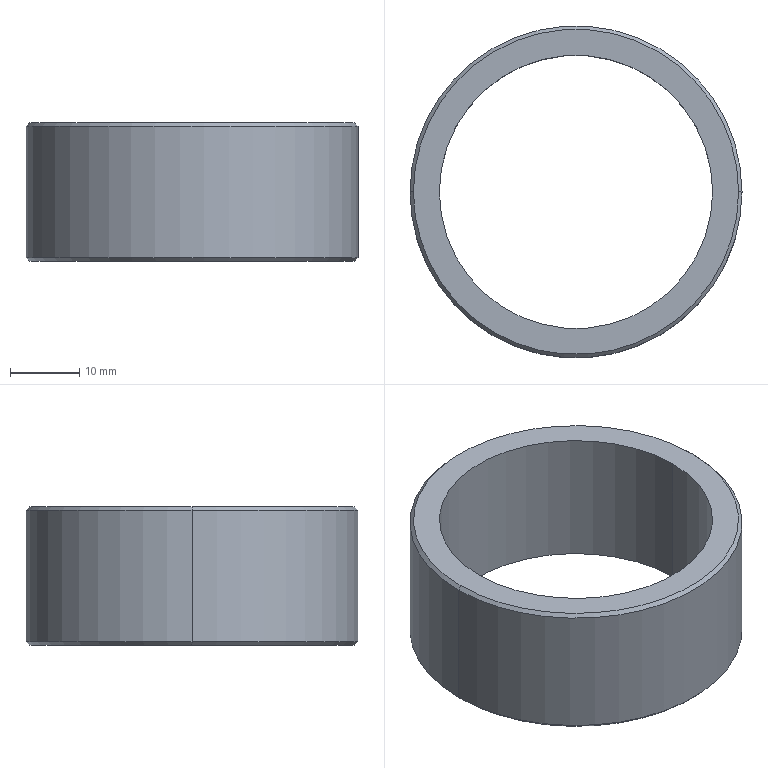Part | SolidWorks | features Chamfer 1, Extrusion 1 | 1 solid | 10 faces | box 48 x 48 x 20 mm | volume 11645 mm3 | cone 4 | cylinder 4 | plane 2 | commonest cylinder face diameters 39.5 x2 48 x2
STEP:
#1=CARTESIAN_POINT('',(23.5,0.,10.));
#2=VERTEX_POINT('',#1);
#3=CARTESIAN_POINT('',(-23.5,0.,10.));
#4=VERTEX_POINT('',#3);
#5=CARTESIAN_POINT('',(0.,0.,10.));
#6=DIRECTION('',(0.,0.,1.));
#7=DIRECTION('',(1.,0.,0.));
#8=AXIS2_PLACEMENT_3D('',#5,#6,#7);
#9=CIRCLE('',#8,23.5);
#10=EDGE_CURVE('',#2,#4,#9,.T.);
#11=ORIENTED_EDGE('',*,*,#10,.F.);
#12=CARTESIAN_POINT('',(24.,0.,9.5));
#13=VERTEX_POINT('',#12);
#14=CARTESIAN_POINT('',(23.5,0.,10.));
#15=DIRECTION('',(0.7071,0.,-0.7071));
#16=VECTOR('',#15,1000.);
#17=LINE('',#14,#16);
#18=EDGE_CURVE('',#2,#13,#17,.T.);
#19=ORIENTED_EDGE('',*,*,#18,.T.);
#20=CARTESIAN_POINT('',(-24.,0.,9.5));
#21=VERTEX_POINT('',#20);
#22=CARTESIAN_POINT('',(0.,0.,9.5));
#23=DIRECTION('',(0.,0.,-1.));
#24=DIRECTION('',(1.,0.,0.));
#25=AXIS2_PLACEMENT_3D('',#22,#23,#24);
#26=CIRCLE('',#25,24.);
#27=EDGE_CURVE('',#21,#13,#26,.T.);
#28=ORIENTED_EDGE('',*,*,#27,.F.);
#29=CARTESIAN_POINT('',(-23.5,0.,10.));
#30=DIRECTION('',(-0.7071,0.,-0.7071));
#31=VECTOR('',#30,1000.);
#32=LINE('',#29,#31);
#33=EDGE_CURVE('',#4,#21,#32,.T.);
#34=ORIENTED_EDGE('',*,*,#33,.F.);
#35=EDGE_LOOP('',(#11,#19,#28,#34));
#36=FACE_OUTER_BOUND('',#35,.T.);
#37=CARTESIAN_POINT('',(0.,0.,10.));
#38=DIRECTION('',(0.,0.,-1.));
#39=DIRECTION('',(-1.,0.,0.));
#40=AXIS2_PLACEMENT_3D('',#37,#38,#39);
#41=CONICAL_SURFACE('',#40,23.5,0.7854);
#42=ADVANCED_FACE('',(#36),#41,.T.);
#43=CARTESIAN_POINT('',(-23.5,0.,-10.));
#44=VERTEX_POINT('',#43);
#45=CARTESIAN_POINT('',(23.5,0.,-10.));
#46=VERTEX_POINT('',#45);
#47=CARTESIAN_POINT('',(0.,0.,-10.));
#48=DIRECTION('',(0.,0.,-1.));
#49=DIRECTION('',(1.,0.,0.));
#50=AXIS2_PLACEMENT_3D('',#47,#48,#49);
#51=CIRCLE('',#50,23.5);
#52=EDGE_CURVE('',#44,#46,#51,.T.);
#53=ORIENTED_EDGE('',*,*,#52,.F.);
#54=CARTESIAN_POINT('',(-24.,0.,-9.5));
#55=VERTEX_POINT('',#54);
#56=CARTESIAN_POINT('',(-24.,0.,-9.5));
#57=DIRECTION('',(-0.7071,0.,0.7071));
#58=VECTOR('',#57,1000.);
#59=LINE('',#56,#58);
#60=EDGE_CURVE('',#44,#55,#59,.T.);
#61=ORIENTED_EDGE('',*,*,#60,.T.);
#62=CARTESIAN_POINT('',(24.,0.,-9.5));
#63=VERTEX_POINT('',#62);
#64=CARTESIAN_POINT('',(0.,0.,-9.5));
#65=DIRECTION('',(0.,0.,1.));
#66=DIRECTION('',(1.,0.,0.));
#67=AXIS2_PLACEMENT_3D('',#64,#65,#66);
#68=CIRCLE('',#67,24.);
#69=EDGE_CURVE('',#63,#55,#68,.T.);
#70=ORIENTED_EDGE('',*,*,#69,.F.);
#71=CARTESIAN_POINT('',(24.,0.,-9.5));
#72=DIRECTION('',(0.7071,0.,0.7071));
#73=VECTOR('',#72,1000.);
#74=LINE('',#71,#73);
#75=EDGE_CURVE('',#46,#63,#74,.T.);
#76=ORIENTED_EDGE('',*,*,#75,.F.);
#77=EDGE_LOOP('',(#53,#61,#70,#76));
#78=FACE_OUTER_BOUND('',#77,.T.);
#79=CARTESIAN_POINT('',(0.,0.,-9.5));
#80=DIRECTION('',(0.,0.,1.));
#81=DIRECTION('',(1.,0.,0.));
#82=AXIS2_PLACEMENT_3D('',#79,#80,#81);
#83=CONICAL_SURFACE('',#82,24.,0.7854);
#84=ADVANCED_FACE('',(#78),#83,.T.);
#85=CARTESIAN_POINT('',(-19.75,0.,10.));
#86=VERTEX_POINT('',#85);
#87=CARTESIAN_POINT('',(19.75,0.,10.));
#88=VERTEX_POINT('',#87);
#89=CARTESIAN_POINT('',(0.,0.,10.));
#90=DIRECTION('',(0.,0.,1.));
#91=DIRECTION('',(1.,0.,0.));
#92=AXIS2_PLACEMENT_3D('',#89,#90,#91);
#93=CIRCLE('',#92,19.75);
#94=EDGE_CURVE('',#86,#88,#93,.T.);
#95=ORIENTED_EDGE('',*,*,#94,.T.);
#96=CARTESIAN_POINT('',(19.75,0.,-10.));
#97=VERTEX_POINT('',#96);
#98=CARTESIAN_POINT('',(19.75,0.,10.));
#99=DIRECTION('',(0.,0.,-1.));
#100=VECTOR('',#99,1000.);
#101=LINE('',#98,#100);
#102=EDGE_CURVE('',#88,#97,#101,.T.);
#103=ORIENTED_EDGE('',*,*,#102,.T.);
#104=CARTESIAN_POINT('',(-19.75,0.,-10.));
#105=VERTEX_POINT('',#104);
#106=CARTESIAN_POINT('',(0.,0.,-10.));
#107=DIRECTION('',(0.,0.,1.));
#108=DIRECTION('',(1.,0.,0.));
#109=AXIS2_PLACEMENT_3D('',#106,#107,#108);
#110=CIRCLE('',#109,19.75);
#111=EDGE_CURVE('',#105,#97,#110,.T.);
#112=ORIENTED_EDGE('',*,*,#111,.F.);
#113=CARTESIAN_POINT('',(-19.75,0.,10.));
#114=DIRECTION('',(0.,0.,-1.));
#115=VECTOR('',#114,1000.);
#116=LINE('',#113,#115);
#117=EDGE_CURVE('',#86,#105,#116,.T.);
#118=ORIENTED_EDGE('',*,*,#117,.F.);
#119=EDGE_LOOP('',(#95,#103,#112,#118));
#120=FACE_OUTER_BOUND('',#119,.T.);
#121=CARTESIAN_POINT('',(0.,0.,10.));
#122=DIRECTION('',(0.,0.,-1.));
#123=DIRECTION('',(-1.,0.,0.));
#124=AXIS2_PLACEMENT_3D('',#121,#122,#123);
#125=CYLINDRICAL_SURFACE('',#124,19.75);
#126=ADVANCED_FACE('',(#120),#125,.F.);
#127=ORIENTED_EDGE('',*,*,#27,.T.);
#128=CARTESIAN_POINT('',(24.,0.,10.));
#129=DIRECTION('',(0.,0.,-1.));
#130=VECTOR('',#129,1000.);
#131=LINE('',#128,#130);
#132=EDGE_CURVE('',#13,#63,#131,.T.);
#133=ORIENTED_EDGE('',*,*,#132,.T.);
#134=ORIENTED_EDGE('',*,*,#69,.T.);
#135=CARTESIAN_POINT('',(-24.,0.,10.));
#136=DIRECTION('',(0.,0.,-1.));
#137=VECTOR('',#136,1000.);
#138=LINE('',#135,#137);
#139=EDGE_CURVE('',#21,#55,#138,.T.);
#140=ORIENTED_EDGE('',*,*,#139,.F.);
#141=EDGE_LOOP('',(#127,#133,#134,#140));
#142=FACE_OUTER_BOUND('',#141,.T.);
#143=CARTESIAN_POINT('',(0.,0.,10.));
#144=DIRECTION('',(0.,0.,-1.));
#145=DIRECTION('',(-1.,0.,0.));
#146=AXIS2_PLACEMENT_3D('',#143,#144,#145);
#147=CYLINDRICAL_SURFACE('',#146,24.);
#148=ADVANCED_FACE('',(#142),#147,.T.);
#149=CARTESIAN_POINT('',(0.,0.,10.));
#150=DIRECTION('',(0.,0.,1.));
#151=DIRECTION('',(1.,0.,0.));
#152=AXIS2_PLACEMENT_3D('',#149,#150,#151);
#153=CIRCLE('',#152,23.5);
#154=EDGE_CURVE('',#4,#2,#153,.T.);
#155=ORIENTED_EDGE('',*,*,#154,.T.);
#156=ORIENTED_EDGE('',*,*,#10,.T.);
#157=EDGE_LOOP('',(#155,#156));
#158=FACE_OUTER_BOUND('',#157,.T.);
#159=ORIENTED_EDGE('',*,*,#94,.F.);
#160=CARTESIAN_POINT('',(0.,0.,10.));
#161=DIRECTION('',(0.,0.,1.));
#162=DIRECTION('',(1.,0.,0.));
#163=AXIS2_PLACEMENT_3D('',#160,#161,#162);
#164=CIRCLE('',#163,19.75);
#165=EDGE_CURVE('',#88,#86,#164,.T.);
#166=ORIENTED_EDGE('',*,*,#165,.F.);
#167=EDGE_LOOP('',(#159,#166));
#168=FACE_BOUND('',#167,.T.);
#169=CARTESIAN_POINT('',(0.,0.,10.));
#170=DIRECTION('',(0.,0.,1.));
#171=DIRECTION('',(1.,0.,0.));
#172=AXIS2_PLACEMENT_3D('',#169,#170,#171);
#173=PLANE('',#172);
#174=ADVANCED_FACE('',(#158,#168),#173,.T.);
#175=CARTESIAN_POINT('',(0.,0.,-10.));
#176=DIRECTION('',(0.,0.,-1.));
#177=DIRECTION('',(1.,0.,0.));
#178=AXIS2_PLACEMENT_3D('',#175,#176,#177);
#179=CIRCLE('',#178,23.5);
#180=EDGE_CURVE('',#46,#44,#179,.T.);
#181=ORIENTED_EDGE('',*,*,#180,.T.);
#182=ORIENTED_EDGE('',*,*,#52,.T.);
#183=EDGE_LOOP('',(#181,#182));
#184=FACE_OUTER_BOUND('',#183,.T.);
#185=ORIENTED_EDGE('',*,*,#111,.T.);
#186=CARTESIAN_POINT('',(0.,0.,-10.));
#187=DIRECTION('',(0.,0.,1.));
#188=DIRECTION('',(1.,0.,0.));
#189=AXIS2_PLACEMENT_3D('',#186,#187,#188);
#190=CIRCLE('',#189,19.75);
#191=EDGE_CURVE('',#97,#105,#190,.T.);
#192=ORIENTED_EDGE('',*,*,#191,.T.);
#193=EDGE_LOOP('',(#185,#192));
#194=FACE_BOUND('',#193,.T.);
#195=CARTESIAN_POINT('',(0.,0.,-10.));
#196=DIRECTION('',(0.,0.,1.));
#197=DIRECTION('',(1.,0.,0.));
#198=AXIS2_PLACEMENT_3D('',#195,#196,#197);
#199=PLANE('',#198);
#200=ADVANCED_FACE('',(#184,#194),#199,.F.);
#201=ORIENTED_EDGE('',*,*,#132,.F.);
#202=CARTESIAN_POINT('',(0.,0.,9.5));
#203=DIRECTION('',(0.,0.,-1.));
#204=DIRECTION('',(1.,0.,0.));
#205=AXIS2_PLACEMENT_3D('',#202,#203,#204);
#206=CIRCLE('',#205,24.);
#207=EDGE_CURVE('',#13,#21,#206,.T.);
#208=ORIENTED_EDGE('',*,*,#207,.T.);
#209=ORIENTED_EDGE('',*,*,#139,.T.);
#210=CARTESIAN_POINT('',(0.,0.,-9.5));
#211=DIRECTION('',(0.,0.,1.));
#212=DIRECTION('',(1.,0.,0.));
#213=AXIS2_PLACEMENT_3D('',#210,#211,#212);
#214=CIRCLE('',#213,24.);
#215=EDGE_CURVE('',#55,#63,#214,.T.);
#216=ORIENTED_EDGE('',*,*,#215,.T.);
#217=EDGE_LOOP('',(#201,#208,#209,#216));
#218=FACE_OUTER_BOUND('',#217,.T.);
#219=CARTESIAN_POINT('',(0.,0.,10.));
#220=DIRECTION('',(0.,0.,-1.));
#221=DIRECTION('',(-1.,0.,0.));
#222=AXIS2_PLACEMENT_3D('',#219,#220,#221);
#223=CYLINDRICAL_SURFACE('',#222,24.);
#224=ADVANCED_FACE('',(#218),#223,.T.);
#225=ORIENTED_EDGE('',*,*,#102,.F.);
#226=ORIENTED_EDGE('',*,*,#165,.T.);
#227=ORIENTED_EDGE('',*,*,#117,.T.);
#228=ORIENTED_EDGE('',*,*,#191,.F.);
#229=EDGE_LOOP('',(#225,#226,#227,#228));
#230=FACE_OUTER_BOUND('',#229,.T.);
#231=CARTESIAN_POINT('',(0.,0.,10.));
#232=DIRECTION('',(0.,0.,-1.));
#233=DIRECTION('',(-1.,0.,0.));
#234=AXIS2_PLACEMENT_3D('',#231,#232,#233);
#235=CYLINDRICAL_SURFACE('',#234,19.75);
#236=ADVANCED_FACE('',(#230),#235,.F.);
#237=ORIENTED_EDGE('',*,*,#60,.F.);
#238=ORIENTED_EDGE('',*,*,#180,.F.);
#239=ORIENTED_EDGE('',*,*,#75,.T.);
#240=ORIENTED_EDGE('',*,*,#215,.F.);
#241=EDGE_LOOP('',(#237,#238,#239,#240));
#242=FACE_OUTER_BOUND('',#241,.T.);
#243=CARTESIAN_POINT('',(0.,0.,-9.5));
#244=DIRECTION('',(0.,0.,1.));
#245=DIRECTION('',(1.,0.,0.));
#246=AXIS2_PLACEMENT_3D('',#243,#244,#245);
#247=CONICAL_SURFACE('',#246,24.,0.7854);
#248=ADVANCED_FACE('',(#242),#247,.T.);
#249=ORIENTED_EDGE('',*,*,#18,.F.);
#250=ORIENTED_EDGE('',*,*,#154,.F.);
#251=ORIENTED_EDGE('',*,*,#33,.T.);
#252=ORIENTED_EDGE('',*,*,#207,.F.);
#253=EDGE_LOOP('',(#249,#250,#251,#252));
#254=FACE_OUTER_BOUND('',#253,.T.);
#255=CARTESIAN_POINT('',(0.,0.,10.));
#256=DIRECTION('',(0.,0.,-1.));
#257=DIRECTION('',(-1.,0.,0.));
#258=AXIS2_PLACEMENT_3D('',#255,#256,#257);
#259=CONICAL_SURFACE('',#258,23.5,0.7854);
#260=ADVANCED_FACE('',(#254),#259,.T.);
#261=CLOSED_SHELL('',(#42,#84,#126,#148,#174,#200,#224,#236,#248,#260));
#262=MANIFOLD_SOLID_BREP('',#261);
#263=CARTESIAN_POINT('',(0.,0.,0.));
#264=DIRECTION('',(0.,0.,1.));
#265=DIRECTION('',(1.,0.,0.));
#266=AXIS2_PLACEMENT_3D('',#263,#264,#265);
#267=(LENGTH_UNIT()NAMED_UNIT(*)SI_UNIT(.MILLI.,.METRE.));
#268=UNCERTAINTY_MEASURE_WITH_UNIT(LENGTH_MEASURE(0.00001),#267,'','');
#269=(NAMED_UNIT(*)PLANE_ANGLE_UNIT()SI_UNIT($,.RADIAN.));
#270=(NAMED_UNIT(*)SI_UNIT($,.STERADIAN.)SOLID_ANGLE_UNIT());
#271=(GEOMETRIC_REPRESENTATION_CONTEXT(3)GLOBAL_UNCERTAINTY_ASSIGNED_CONTEXT((#268))GLOBAL_UNIT_ASSIGNED_CONTEXT((#267,#269,#270))REPRESENTATION_CONTEXT('',''));
#272=ADVANCED_BREP_SHAPE_REPRESENTATION('',(#262,#266),#271);